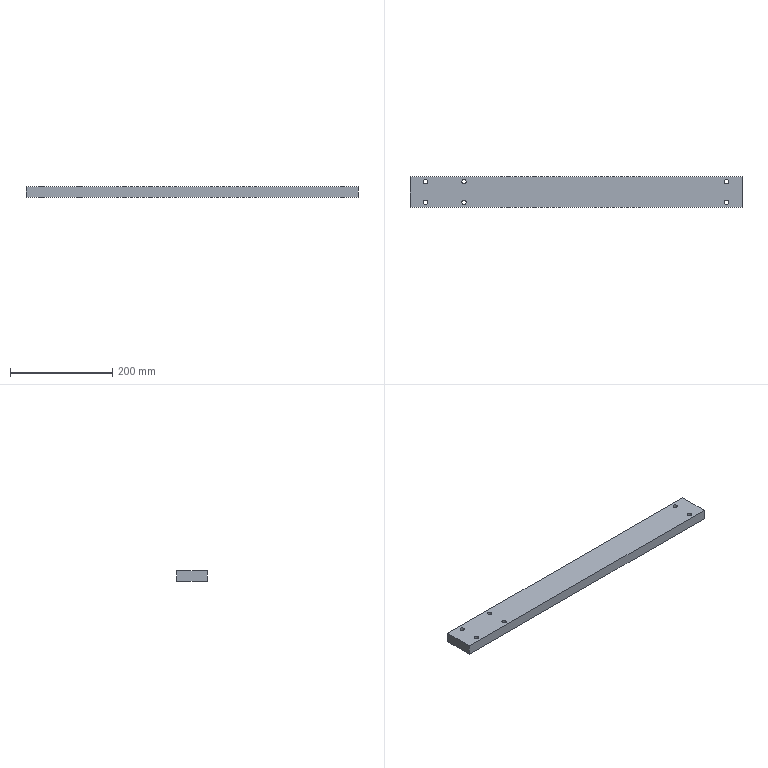Part | STEP file | JBJ-P-1006-02 | 1 solid | 12 faces | box 648 x 60 x 20 mm | volume 770791 mm3 | plane 6 | cylinder 6 | commonest cylinder face diameters 8.5 x6
STEP:
#1=CARTESIAN_POINT('',(0.,0.,0.));
#2=VERTEX_POINT('',#1);
#3=CARTESIAN_POINT('',(648.,0.,0.));
#4=VERTEX_POINT('',#3);
#5=CARTESIAN_POINT('',(0.,0.,0.));
#6=DIRECTION('',(1.,0.,0.));
#7=VECTOR('',#6,1000.);
#8=LINE('',#5,#7);
#9=EDGE_CURVE('',#2,#4,#8,.T.);
#10=ORIENTED_EDGE('',*,*,#9,.F.);
#11=CARTESIAN_POINT('',(0.,0.,20.));
#12=VERTEX_POINT('',#11);
#13=CARTESIAN_POINT('',(0.,0.,20.));
#14=DIRECTION('',(0.,0.,-1.));
#15=VECTOR('',#14,1000.);
#16=LINE('',#13,#15);
#17=EDGE_CURVE('',#12,#2,#16,.T.);
#18=ORIENTED_EDGE('',*,*,#17,.F.);
#19=CARTESIAN_POINT('',(648.,0.,20.));
#20=VERTEX_POINT('',#19);
#21=CARTESIAN_POINT('',(0.,0.,20.));
#22=DIRECTION('',(1.,0.,0.));
#23=VECTOR('',#22,1000.);
#24=LINE('',#21,#23);
#25=EDGE_CURVE('',#12,#20,#24,.T.);
#26=ORIENTED_EDGE('',*,*,#25,.T.);
#27=CARTESIAN_POINT('',(648.,0.,20.));
#28=DIRECTION('',(0.,0.,-1.));
#29=VECTOR('',#28,1000.);
#30=LINE('',#27,#29);
#31=EDGE_CURVE('',#20,#4,#30,.T.);
#32=ORIENTED_EDGE('',*,*,#31,.T.);
#33=EDGE_LOOP('',(#10,#18,#26,#32));
#34=FACE_OUTER_BOUND('',#33,.T.);
#35=CARTESIAN_POINT('',(0.,0.,20.));
#36=DIRECTION('',(0.,1.,0.));
#37=DIRECTION('',(0.,0.,1.));
#38=AXIS2_PLACEMENT_3D('',#35,#36,#37);
#39=PLANE('',#38);
#40=ADVANCED_FACE('',(#34),#39,.T.);
#41=CARTESIAN_POINT('',(0.,-60.,0.));
#42=VERTEX_POINT('',#41);
#43=CARTESIAN_POINT('',(0.,0.,0.));
#44=DIRECTION('',(0.,-1.,0.));
#45=VECTOR('',#44,1000.);
#46=LINE('',#43,#45);
#47=EDGE_CURVE('',#2,#42,#46,.T.);
#48=ORIENTED_EDGE('',*,*,#47,.T.);
#49=CARTESIAN_POINT('',(0.,-60.,20.));
#50=VERTEX_POINT('',#49);
#51=CARTESIAN_POINT('',(0.,-60.,20.));
#52=DIRECTION('',(0.,0.,-1.));
#53=VECTOR('',#52,1000.);
#54=LINE('',#51,#53);
#55=EDGE_CURVE('',#50,#42,#54,.T.);
#56=ORIENTED_EDGE('',*,*,#55,.F.);
#57=CARTESIAN_POINT('',(0.,0.,20.));
#58=DIRECTION('',(0.,-1.,0.));
#59=VECTOR('',#58,1000.);
#60=LINE('',#57,#59);
#61=EDGE_CURVE('',#12,#50,#60,.T.);
#62=ORIENTED_EDGE('',*,*,#61,.F.);
#63=ORIENTED_EDGE('',*,*,#17,.T.);
#64=EDGE_LOOP('',(#48,#56,#62,#63));
#65=FACE_OUTER_BOUND('',#64,.T.);
#66=CARTESIAN_POINT('',(0.,0.,20.));
#67=DIRECTION('',(1.,0.,0.));
#68=DIRECTION('',(0.,0.,-1.));
#69=AXIS2_PLACEMENT_3D('',#66,#67,#68);
#70=PLANE('',#69);
#71=ADVANCED_FACE('',(#65),#70,.F.);
#72=CARTESIAN_POINT('',(648.,-60.,0.));
#73=VERTEX_POINT('',#72);
#74=CARTESIAN_POINT('',(0.,-60.,0.));
#75=DIRECTION('',(1.,0.,0.));
#76=VECTOR('',#75,1000.);
#77=LINE('',#74,#76);
#78=EDGE_CURVE('',#42,#73,#77,.T.);
#79=ORIENTED_EDGE('',*,*,#78,.T.);
#80=CARTESIAN_POINT('',(648.,-60.,20.));
#81=VERTEX_POINT('',#80);
#82=CARTESIAN_POINT('',(648.,-60.,20.));
#83=DIRECTION('',(0.,0.,-1.));
#84=VECTOR('',#83,1000.);
#85=LINE('',#82,#84);
#86=EDGE_CURVE('',#81,#73,#85,.T.);
#87=ORIENTED_EDGE('',*,*,#86,.F.);
#88=CARTESIAN_POINT('',(0.,-60.,20.));
#89=DIRECTION('',(1.,0.,0.));
#90=VECTOR('',#89,1000.);
#91=LINE('',#88,#90);
#92=EDGE_CURVE('',#50,#81,#91,.T.);
#93=ORIENTED_EDGE('',*,*,#92,.F.);
#94=ORIENTED_EDGE('',*,*,#55,.T.);
#95=EDGE_LOOP('',(#79,#87,#93,#94));
#96=FACE_OUTER_BOUND('',#95,.T.);
#97=CARTESIAN_POINT('',(0.,-60.,20.));
#98=DIRECTION('',(0.,1.,0.));
#99=DIRECTION('',(0.,0.,1.));
#100=AXIS2_PLACEMENT_3D('',#97,#98,#99);
#101=PLANE('',#100);
#102=ADVANCED_FACE('',(#96),#101,.F.);
#103=CARTESIAN_POINT('',(648.,0.,0.));
#104=DIRECTION('',(0.,-1.,0.));
#105=VECTOR('',#104,1000.);
#106=LINE('',#103,#105);
#107=EDGE_CURVE('',#4,#73,#106,.T.);
#108=ORIENTED_EDGE('',*,*,#107,.F.);
#109=ORIENTED_EDGE('',*,*,#31,.F.);
#110=CARTESIAN_POINT('',(648.,0.,20.));
#111=DIRECTION('',(0.,-1.,0.));
#112=VECTOR('',#111,1000.);
#113=LINE('',#110,#112);
#114=EDGE_CURVE('',#20,#81,#113,.T.);
#115=ORIENTED_EDGE('',*,*,#114,.T.);
#116=ORIENTED_EDGE('',*,*,#86,.T.);
#117=EDGE_LOOP('',(#108,#109,#115,#116));
#118=FACE_OUTER_BOUND('',#117,.T.);
#119=CARTESIAN_POINT('',(648.,0.,20.));
#120=DIRECTION('',(1.,0.,0.));
#121=DIRECTION('',(0.,0.,-1.));
#122=AXIS2_PLACEMENT_3D('',#119,#120,#121);
#123=PLANE('',#122);
#124=ADVANCED_FACE('',(#118),#123,.T.);
#125=CARTESIAN_POINT('',(109.75,-10.,20.));
#126=VERTEX_POINT('',#125);
#127=CARTESIAN_POINT('',(105.5,-10.,20.));
#128=DIRECTION('',(0.,0.,1.));
#129=DIRECTION('',(1.,0.,0.));
#130=AXIS2_PLACEMENT_3D('',#127,#128,#129);
#131=CIRCLE('',#130,4.25);
#132=EDGE_CURVE('',#126,#126,#131,.T.);
#133=ORIENTED_EDGE('',*,*,#132,.F.);
#134=EDGE_LOOP('',(#133));
#135=FACE_BOUND('',#134,.T.);
#136=CARTESIAN_POINT('',(109.75,-50.,20.));
#137=VERTEX_POINT('',#136);
#138=CARTESIAN_POINT('',(105.5,-50.,20.));
#139=DIRECTION('',(0.,0.,1.));
#140=DIRECTION('',(1.,0.,0.));
#141=AXIS2_PLACEMENT_3D('',#138,#139,#140);
#142=CIRCLE('',#141,4.25);
#143=EDGE_CURVE('',#137,#137,#142,.T.);
#144=ORIENTED_EDGE('',*,*,#143,.F.);
#145=EDGE_LOOP('',(#144));
#146=FACE_BOUND('',#145,.T.);
#147=CARTESIAN_POINT('',(34.25,-50.,20.));
#148=VERTEX_POINT('',#147);
#149=CARTESIAN_POINT('',(30.,-50.,20.));
#150=DIRECTION('',(0.,0.,1.));
#151=DIRECTION('',(1.,0.,0.));
#152=AXIS2_PLACEMENT_3D('',#149,#150,#151);
#153=CIRCLE('',#152,4.25);
#154=EDGE_CURVE('',#148,#148,#153,.T.);
#155=ORIENTED_EDGE('',*,*,#154,.F.);
#156=EDGE_LOOP('',(#155));
#157=FACE_BOUND('',#156,.T.);
#158=CARTESIAN_POINT('',(34.25,-10.,20.));
#159=VERTEX_POINT('',#158);
#160=CARTESIAN_POINT('',(30.,-10.,20.));
#161=DIRECTION('',(0.,0.,1.));
#162=DIRECTION('',(1.,0.,0.));
#163=AXIS2_PLACEMENT_3D('',#160,#161,#162);
#164=CIRCLE('',#163,4.25);
#165=EDGE_CURVE('',#159,#159,#164,.T.);
#166=ORIENTED_EDGE('',*,*,#165,.F.);
#167=EDGE_LOOP('',(#166));
#168=FACE_BOUND('',#167,.T.);
#169=CARTESIAN_POINT('',(622.25,-10.,20.));
#170=VERTEX_POINT('',#169);
#171=CARTESIAN_POINT('',(618.,-10.,20.));
#172=DIRECTION('',(0.,0.,1.));
#173=DIRECTION('',(1.,0.,0.));
#174=AXIS2_PLACEMENT_3D('',#171,#172,#173);
#175=CIRCLE('',#174,4.25);
#176=EDGE_CURVE('',#170,#170,#175,.T.);
#177=ORIENTED_EDGE('',*,*,#176,.F.);
#178=EDGE_LOOP('',(#177));
#179=FACE_BOUND('',#178,.T.);
#180=CARTESIAN_POINT('',(622.25,-50.,20.));
#181=VERTEX_POINT('',#180);
#182=CARTESIAN_POINT('',(618.,-50.,20.));
#183=DIRECTION('',(0.,0.,1.));
#184=DIRECTION('',(1.,0.,0.));
#185=AXIS2_PLACEMENT_3D('',#182,#183,#184);
#186=CIRCLE('',#185,4.25);
#187=EDGE_CURVE('',#181,#181,#186,.T.);
#188=ORIENTED_EDGE('',*,*,#187,.F.);
#189=EDGE_LOOP('',(#188));
#190=FACE_BOUND('',#189,.T.);
#191=ORIENTED_EDGE('',*,*,#25,.F.);
#192=ORIENTED_EDGE('',*,*,#61,.T.);
#193=ORIENTED_EDGE('',*,*,#92,.T.);
#194=ORIENTED_EDGE('',*,*,#114,.F.);
#195=EDGE_LOOP('',(#191,#192,#193,#194));
#196=FACE_OUTER_BOUND('',#195,.T.);
#197=CARTESIAN_POINT('',(0.,0.,20.));
#198=DIRECTION('',(0.,0.,-1.));
#199=DIRECTION('',(-1.,0.,0.));
#200=AXIS2_PLACEMENT_3D('',#197,#198,#199);
#201=PLANE('',#200);
#202=ADVANCED_FACE('',(#135,#146,#157,#168,#179,#190,#196),#201,.F.);
#203=CARTESIAN_POINT('',(109.75,-10.,0.));
#204=VERTEX_POINT('',#203);
#205=CARTESIAN_POINT('',(105.5,-10.,0.));
#206=DIRECTION('',(0.,0.,1.));
#207=DIRECTION('',(1.,0.,0.));
#208=AXIS2_PLACEMENT_3D('',#205,#206,#207);
#209=CIRCLE('',#208,4.25);
#210=EDGE_CURVE('',#204,#204,#209,.T.);
#211=ORIENTED_EDGE('',*,*,#210,.T.);
#212=EDGE_LOOP('',(#211));
#213=FACE_BOUND('',#212,.T.);
#214=CARTESIAN_POINT('',(109.75,-50.,0.));
#215=VERTEX_POINT('',#214);
#216=CARTESIAN_POINT('',(105.5,-50.,0.));
#217=DIRECTION('',(0.,0.,1.));
#218=DIRECTION('',(1.,0.,0.));
#219=AXIS2_PLACEMENT_3D('',#216,#217,#218);
#220=CIRCLE('',#219,4.25);
#221=EDGE_CURVE('',#215,#215,#220,.T.);
#222=ORIENTED_EDGE('',*,*,#221,.T.);
#223=EDGE_LOOP('',(#222));
#224=FACE_BOUND('',#223,.T.);
#225=CARTESIAN_POINT('',(34.25,-50.,0.));
#226=VERTEX_POINT('',#225);
#227=CARTESIAN_POINT('',(30.,-50.,0.));
#228=DIRECTION('',(0.,0.,1.));
#229=DIRECTION('',(1.,0.,0.));
#230=AXIS2_PLACEMENT_3D('',#227,#228,#229);
#231=CIRCLE('',#230,4.25);
#232=EDGE_CURVE('',#226,#226,#231,.T.);
#233=ORIENTED_EDGE('',*,*,#232,.T.);
#234=EDGE_LOOP('',(#233));
#235=FACE_BOUND('',#234,.T.);
#236=CARTESIAN_POINT('',(34.25,-10.,0.));
#237=VERTEX_POINT('',#236);
#238=CARTESIAN_POINT('',(30.,-10.,0.));
#239=DIRECTION('',(0.,0.,1.));
#240=DIRECTION('',(1.,0.,0.));
#241=AXIS2_PLACEMENT_3D('',#238,#239,#240);
#242=CIRCLE('',#241,4.25);
#243=EDGE_CURVE('',#237,#237,#242,.T.);
#244=ORIENTED_EDGE('',*,*,#243,.T.);
#245=EDGE_LOOP('',(#244));
#246=FACE_BOUND('',#245,.T.);
#247=CARTESIAN_POINT('',(622.25,-10.,0.));
#248=VERTEX_POINT('',#247);
#249=CARTESIAN_POINT('',(618.,-10.,0.));
#250=DIRECTION('',(0.,0.,1.));
#251=DIRECTION('',(1.,0.,0.));
#252=AXIS2_PLACEMENT_3D('',#249,#250,#251);
#253=CIRCLE('',#252,4.25);
#254=EDGE_CURVE('',#248,#248,#253,.T.);
#255=ORIENTED_EDGE('',*,*,#254,.T.);
#256=EDGE_LOOP('',(#255));
#257=FACE_BOUND('',#256,.T.);
#258=CARTESIAN_POINT('',(622.25,-50.,0.));
#259=VERTEX_POINT('',#258);
#260=CARTESIAN_POINT('',(618.,-50.,0.));
#261=DIRECTION('',(0.,0.,1.));
#262=DIRECTION('',(1.,0.,0.));
#263=AXIS2_PLACEMENT_3D('',#260,#261,#262);
#264=CIRCLE('',#263,4.25);
#265=EDGE_CURVE('',#259,#259,#264,.T.);
#266=ORIENTED_EDGE('',*,*,#265,.T.);
#267=EDGE_LOOP('',(#266));
#268=FACE_BOUND('',#267,.T.);
#269=ORIENTED_EDGE('',*,*,#9,.T.);
#270=ORIENTED_EDGE('',*,*,#107,.T.);
#271=ORIENTED_EDGE('',*,*,#78,.F.);
#272=ORIENTED_EDGE('',*,*,#47,.F.);
#273=EDGE_LOOP('',(#269,#270,#271,#272));
#274=FACE_OUTER_BOUND('',#273,.T.);
#275=CARTESIAN_POINT('',(0.,0.,0.));
#276=DIRECTION('',(0.,0.,-1.));
#277=DIRECTION('',(-1.,0.,0.));
#278=AXIS2_PLACEMENT_3D('',#275,#276,#277);
#279=PLANE('',#278);
#280=ADVANCED_FACE('',(#213,#224,#235,#246,#257,#268,#274),#279,.T.);
#281=ORIENTED_EDGE('',*,*,#265,.F.);
#282=EDGE_LOOP('',(#281));
#283=FACE_OUTER_BOUND('',#282,.T.);
#284=ORIENTED_EDGE('',*,*,#187,.T.);
#285=EDGE_LOOP('',(#284));
#286=FACE_OUTER_BOUND('',#285,.T.);
#287=CARTESIAN_POINT('',(618.,-50.,20.));
#288=DIRECTION('',(0.,0.,1.));
#289=DIRECTION('',(1.,0.,0.));
#290=AXIS2_PLACEMENT_3D('',#287,#288,#289);
#291=CYLINDRICAL_SURFACE('',#290,4.25);
#292=ADVANCED_FACE('',(#283,#286),#291,.F.);
#293=ORIENTED_EDGE('',*,*,#254,.F.);
#294=EDGE_LOOP('',(#293));
#295=FACE_OUTER_BOUND('',#294,.T.);
#296=ORIENTED_EDGE('',*,*,#176,.T.);
#297=EDGE_LOOP('',(#296));
#298=FACE_OUTER_BOUND('',#297,.T.);
#299=CARTESIAN_POINT('',(618.,-10.,20.));
#300=DIRECTION('',(0.,0.,1.));
#301=DIRECTION('',(1.,0.,0.));
#302=AXIS2_PLACEMENT_3D('',#299,#300,#301);
#303=CYLINDRICAL_SURFACE('',#302,4.25);
#304=ADVANCED_FACE('',(#295,#298),#303,.F.);
#305=ORIENTED_EDGE('',*,*,#243,.F.);
#306=EDGE_LOOP('',(#305));
#307=FACE_OUTER_BOUND('',#306,.T.);
#308=ORIENTED_EDGE('',*,*,#165,.T.);
#309=EDGE_LOOP('',(#308));
#310=FACE_OUTER_BOUND('',#309,.T.);
#311=CARTESIAN_POINT('',(30.,-10.,20.));
#312=DIRECTION('',(0.,0.,1.));
#313=DIRECTION('',(1.,0.,0.));
#314=AXIS2_PLACEMENT_3D('',#311,#312,#313);
#315=CYLINDRICAL_SURFACE('',#314,4.25);
#316=ADVANCED_FACE('',(#307,#310),#315,.F.);
#317=ORIENTED_EDGE('',*,*,#232,.F.);
#318=EDGE_LOOP('',(#317));
#319=FACE_OUTER_BOUND('',#318,.T.);
#320=ORIENTED_EDGE('',*,*,#154,.T.);
#321=EDGE_LOOP('',(#320));
#322=FACE_OUTER_BOUND('',#321,.T.);
#323=CARTESIAN_POINT('',(30.,-50.,20.));
#324=DIRECTION('',(0.,0.,1.));
#325=DIRECTION('',(1.,0.,0.));
#326=AXIS2_PLACEMENT_3D('',#323,#324,#325);
#327=CYLINDRICAL_SURFACE('',#326,4.25);
#328=ADVANCED_FACE('',(#319,#322),#327,.F.);
#329=ORIENTED_EDGE('',*,*,#221,.F.);
#330=EDGE_LOOP('',(#329));
#331=FACE_OUTER_BOUND('',#330,.T.);
#332=ORIENTED_EDGE('',*,*,#143,.T.);
#333=EDGE_LOOP('',(#332));
#334=FACE_OUTER_BOUND('',#333,.T.);
#335=CARTESIAN_POINT('',(105.5,-50.,20.));
#336=DIRECTION('',(0.,0.,1.));
#337=DIRECTION('',(1.,0.,0.));
#338=AXIS2_PLACEMENT_3D('',#335,#336,#337);
#339=CYLINDRICAL_SURFACE('',#338,4.25);
#340=ADVANCED_FACE('',(#331,#334),#339,.F.);
#341=ORIENTED_EDGE('',*,*,#210,.F.);
#342=EDGE_LOOP('',(#341));
#343=FACE_OUTER_BOUND('',#342,.T.);
#344=ORIENTED_EDGE('',*,*,#132,.T.);
#345=EDGE_LOOP('',(#344));
#346=FACE_OUTER_BOUND('',#345,.T.);
#347=CARTESIAN_POINT('',(105.5,-10.,20.));
#348=DIRECTION('',(0.,0.,1.));
#349=DIRECTION('',(1.,0.,0.));
#350=AXIS2_PLACEMENT_3D('',#347,#348,#349);
#351=CYLINDRICAL_SURFACE('',#350,4.25);
#352=ADVANCED_FACE('',(#343,#346),#351,.F.);
#353=CLOSED_SHELL('',(#40,#71,#102,#124,#202,#280,#292,#304,#316,#328,#340,#352));
#354=MANIFOLD_SOLID_BREP('',#353);
#355=CARTESIAN_POINT('',(0.,0.,0.));
#356=DIRECTION('',(0.,0.,1.));
#357=DIRECTION('',(1.,0.,0.));
#358=AXIS2_PLACEMENT_3D('',#355,#356,#357);
#359=(LENGTH_UNIT()NAMED_UNIT(*)SI_UNIT(.MILLI.,.METRE.));
#360=UNCERTAINTY_MEASURE_WITH_UNIT(LENGTH_MEASURE(0.00001),#359,'','');
#361=(NAMED_UNIT(*)PLANE_ANGLE_UNIT()SI_UNIT($,.RADIAN.));
#362=(NAMED_UNIT(*)SI_UNIT($,.STERADIAN.)SOLID_ANGLE_UNIT());
#363=(GEOMETRIC_REPRESENTATION_CONTEXT(3)GLOBAL_UNCERTAINTY_ASSIGNED_CONTEXT((#360))GLOBAL_UNIT_ASSIGNED_CONTEXT((#359,#361,#362))REPRESENTATION_CONTEXT('',''));
#364=ADVANCED_BREP_SHAPE_REPRESENTATION('',(#354,#358),#363);